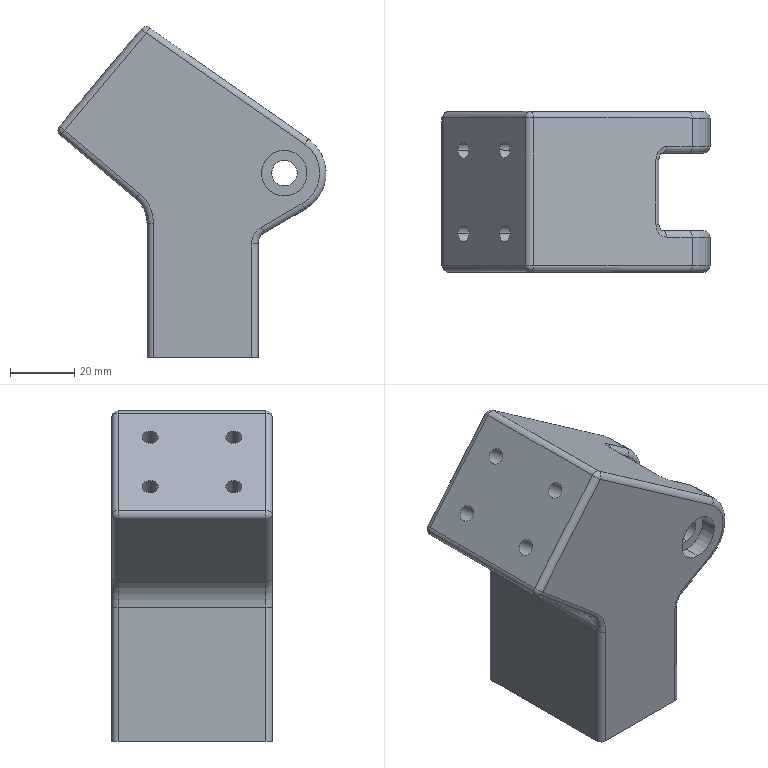Part | SolidWorks | features BaseBody 1 | 1 solid | 128 faces | box 83.451 x 50 x 102.866 mm | volume 198028 mm3 | cylinder 63 | cone 24 | plane 21 | torus 10 | sphere 6 | spline 4 | commonest cylinder face diameters 4 x26 5 x8 5.2 x8 6.8 x8 7.95 x4 14.2 x4